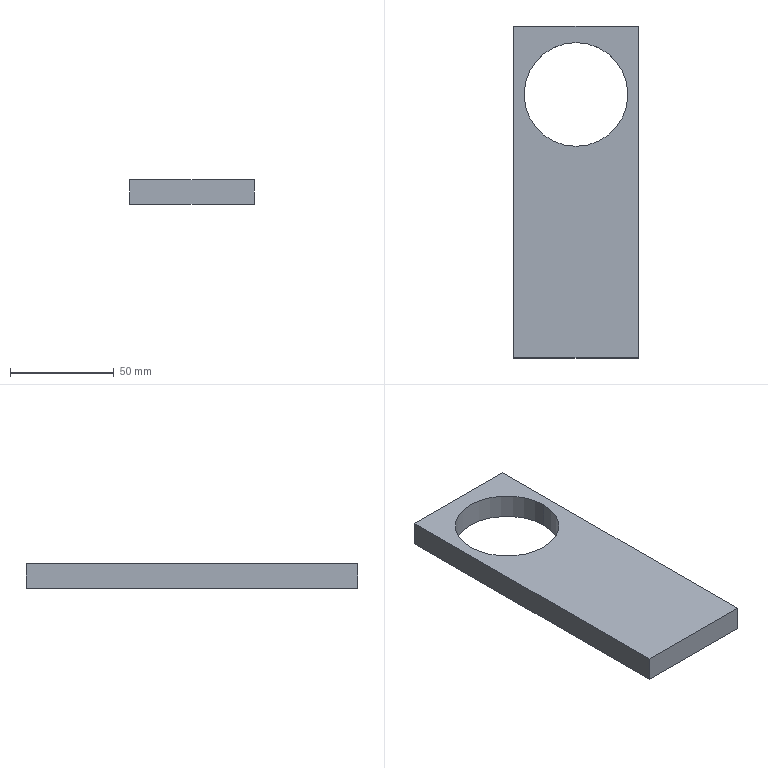Part | SolidWorks | features Extrusion 1, ICE 1 | 1 solid | 8 faces | box 60 x 160 x 12 mm | volume 91638 mm3 | plane 6 | cylinder 2 | commonest cylinder face diameters 50 x2
STEP:
#1=CARTESIAN_POINT('',(-25.,47.,0.));
#2=VERTEX_POINT('',#1);
#3=CARTESIAN_POINT('',(25.,47.,0.));
#4=VERTEX_POINT('',#3);
#5=CARTESIAN_POINT('',(0.,47.,0.));
#6=DIRECTION('',(0.,0.,1.));
#7=DIRECTION('',(1.,0.,0.));
#8=AXIS2_PLACEMENT_3D('',#5,#6,#7);
#9=CIRCLE('',#8,25.);
#10=EDGE_CURVE('',#2,#4,#9,.T.);
#11=ORIENTED_EDGE('',*,*,#10,.F.);
#12=CARTESIAN_POINT('',(-25.,47.,12.));
#13=VERTEX_POINT('',#12);
#14=CARTESIAN_POINT('',(-25.,47.,0.));
#15=DIRECTION('',(0.,0.,1.));
#16=VECTOR('',#15,1000.);
#17=LINE('',#14,#16);
#18=EDGE_CURVE('',#2,#13,#17,.T.);
#19=ORIENTED_EDGE('',*,*,#18,.T.);
#20=CARTESIAN_POINT('',(25.,47.,12.));
#21=VERTEX_POINT('',#20);
#22=CARTESIAN_POINT('',(0.,47.,12.));
#23=DIRECTION('',(0.,0.,1.));
#24=DIRECTION('',(1.,0.,0.));
#25=AXIS2_PLACEMENT_3D('',#22,#23,#24);
#26=CIRCLE('',#25,25.);
#27=EDGE_CURVE('',#13,#21,#26,.T.);
#28=ORIENTED_EDGE('',*,*,#27,.T.);
#29=CARTESIAN_POINT('',(25.,47.,0.));
#30=DIRECTION('',(0.,0.,1.));
#31=VECTOR('',#30,1000.);
#32=LINE('',#29,#31);
#33=EDGE_CURVE('',#4,#21,#32,.T.);
#34=ORIENTED_EDGE('',*,*,#33,.F.);
#35=EDGE_LOOP('',(#11,#19,#28,#34));
#36=FACE_OUTER_BOUND('',#35,.T.);
#37=CARTESIAN_POINT('',(0.,47.,0.));
#38=DIRECTION('',(0.,0.,1.));
#39=DIRECTION('',(1.,0.,0.));
#40=AXIS2_PLACEMENT_3D('',#37,#38,#39);
#41=CYLINDRICAL_SURFACE('',#40,25.);
#42=ADVANCED_FACE('',(#36),#41,.F.);
#43=CARTESIAN_POINT('',(30.,-80.,0.));
#44=VERTEX_POINT('',#43);
#45=CARTESIAN_POINT('',(30.,80.,0.));
#46=VERTEX_POINT('',#45);
#47=CARTESIAN_POINT('',(30.,-80.,0.));
#48=DIRECTION('',(0.,1.,0.));
#49=VECTOR('',#48,1000.);
#50=LINE('',#47,#49);
#51=EDGE_CURVE('',#44,#46,#50,.T.);
#52=ORIENTED_EDGE('',*,*,#51,.T.);
#53=CARTESIAN_POINT('',(30.,80.,12.));
#54=VERTEX_POINT('',#53);
#55=CARTESIAN_POINT('',(30.,80.,12.));
#56=DIRECTION('',(0.,0.,-1.));
#57=VECTOR('',#56,1000.);
#58=LINE('',#55,#57);
#59=EDGE_CURVE('',#54,#46,#58,.T.);
#60=ORIENTED_EDGE('',*,*,#59,.F.);
#61=CARTESIAN_POINT('',(30.,-80.,12.));
#62=VERTEX_POINT('',#61);
#63=CARTESIAN_POINT('',(30.,-80.,12.));
#64=DIRECTION('',(0.,1.,0.));
#65=VECTOR('',#64,1000.);
#66=LINE('',#63,#65);
#67=EDGE_CURVE('',#62,#54,#66,.T.);
#68=ORIENTED_EDGE('',*,*,#67,.F.);
#69=CARTESIAN_POINT('',(30.,-80.,12.));
#70=DIRECTION('',(0.,0.,-1.));
#71=VECTOR('',#70,1000.);
#72=LINE('',#69,#71);
#73=EDGE_CURVE('',#62,#44,#72,.T.);
#74=ORIENTED_EDGE('',*,*,#73,.T.);
#75=EDGE_LOOP('',(#52,#60,#68,#74));
#76=FACE_OUTER_BOUND('',#75,.T.);
#77=CARTESIAN_POINT('',(30.,-80.,12.));
#78=DIRECTION('',(-1.,0.,0.));
#79=DIRECTION('',(0.,0.,1.));
#80=AXIS2_PLACEMENT_3D('',#77,#78,#79);
#81=PLANE('',#80);
#82=ADVANCED_FACE('',(#76),#81,.F.);
#83=CARTESIAN_POINT('',(-30.,80.,0.));
#84=VERTEX_POINT('',#83);
#85=CARTESIAN_POINT('',(-30.,80.,0.));
#86=DIRECTION('',(-1.,0.,0.));
#87=VECTOR('',#86,1000.);
#88=LINE('',#85,#87);
#89=EDGE_CURVE('',#46,#84,#88,.T.);
#90=ORIENTED_EDGE('',*,*,#89,.T.);
#91=CARTESIAN_POINT('',(-30.,80.,12.));
#92=VERTEX_POINT('',#91);
#93=CARTESIAN_POINT('',(-30.,80.,12.));
#94=DIRECTION('',(0.,0.,-1.));
#95=VECTOR('',#94,1000.);
#96=LINE('',#93,#95);
#97=EDGE_CURVE('',#92,#84,#96,.T.);
#98=ORIENTED_EDGE('',*,*,#97,.F.);
#99=CARTESIAN_POINT('',(-30.,80.,12.));
#100=DIRECTION('',(-1.,0.,0.));
#101=VECTOR('',#100,1000.);
#102=LINE('',#99,#101);
#103=EDGE_CURVE('',#54,#92,#102,.T.);
#104=ORIENTED_EDGE('',*,*,#103,.F.);
#105=ORIENTED_EDGE('',*,*,#59,.T.);
#106=EDGE_LOOP('',(#90,#98,#104,#105));
#107=FACE_OUTER_BOUND('',#106,.T.);
#108=CARTESIAN_POINT('',(-30.,80.,12.));
#109=DIRECTION('',(0.,-1.,0.));
#110=DIRECTION('',(0.,0.,-1.));
#111=AXIS2_PLACEMENT_3D('',#108,#109,#110);
#112=PLANE('',#111);
#113=ADVANCED_FACE('',(#107),#112,.F.);
#114=CARTESIAN_POINT('',(-30.,-80.,0.));
#115=VERTEX_POINT('',#114);
#116=CARTESIAN_POINT('',(-30.,-80.,0.));
#117=DIRECTION('',(0.,-1.,0.));
#118=VECTOR('',#117,1000.);
#119=LINE('',#116,#118);
#120=EDGE_CURVE('',#84,#115,#119,.T.);
#121=ORIENTED_EDGE('',*,*,#120,.T.);
#122=CARTESIAN_POINT('',(-30.,-80.,12.));
#123=VERTEX_POINT('',#122);
#124=CARTESIAN_POINT('',(-30.,-80.,12.));
#125=DIRECTION('',(0.,0.,-1.));
#126=VECTOR('',#125,1000.);
#127=LINE('',#124,#126);
#128=EDGE_CURVE('',#123,#115,#127,.T.);
#129=ORIENTED_EDGE('',*,*,#128,.F.);
#130=CARTESIAN_POINT('',(-30.,-80.,12.));
#131=DIRECTION('',(0.,-1.,0.));
#132=VECTOR('',#131,1000.);
#133=LINE('',#130,#132);
#134=EDGE_CURVE('',#92,#123,#133,.T.);
#135=ORIENTED_EDGE('',*,*,#134,.F.);
#136=ORIENTED_EDGE('',*,*,#97,.T.);
#137=EDGE_LOOP('',(#121,#129,#135,#136));
#138=FACE_OUTER_BOUND('',#137,.T.);
#139=CARTESIAN_POINT('',(-30.,-80.,12.));
#140=DIRECTION('',(1.,0.,0.));
#141=DIRECTION('',(0.,0.,-1.));
#142=AXIS2_PLACEMENT_3D('',#139,#140,#141);
#143=PLANE('',#142);
#144=ADVANCED_FACE('',(#138),#143,.F.);
#145=CARTESIAN_POINT('',(-30.,-80.,0.));
#146=DIRECTION('',(1.,0.,0.));
#147=VECTOR('',#146,1000.);
#148=LINE('',#145,#147);
#149=EDGE_CURVE('',#115,#44,#148,.T.);
#150=ORIENTED_EDGE('',*,*,#149,.T.);
#151=ORIENTED_EDGE('',*,*,#73,.F.);
#152=CARTESIAN_POINT('',(-30.,-80.,12.));
#153=DIRECTION('',(1.,0.,0.));
#154=VECTOR('',#153,1000.);
#155=LINE('',#152,#154);
#156=EDGE_CURVE('',#123,#62,#155,.T.);
#157=ORIENTED_EDGE('',*,*,#156,.F.);
#158=ORIENTED_EDGE('',*,*,#128,.T.);
#159=EDGE_LOOP('',(#150,#151,#157,#158));
#160=FACE_OUTER_BOUND('',#159,.T.);
#161=CARTESIAN_POINT('',(-30.,-80.,12.));
#162=DIRECTION('',(0.,1.,0.));
#163=DIRECTION('',(0.,0.,1.));
#164=AXIS2_PLACEMENT_3D('',#161,#162,#163);
#165=PLANE('',#164);
#166=ADVANCED_FACE('',(#160),#165,.F.);
#167=CARTESIAN_POINT('',(0.,47.,12.));
#168=DIRECTION('',(0.,0.,1.));
#169=DIRECTION('',(1.,0.,0.));
#170=AXIS2_PLACEMENT_3D('',#167,#168,#169);
#171=CIRCLE('',#170,25.);
#172=EDGE_CURVE('',#21,#13,#171,.T.);
#173=ORIENTED_EDGE('',*,*,#172,.F.);
#174=ORIENTED_EDGE('',*,*,#27,.F.);
#175=EDGE_LOOP('',(#173,#174));
#176=FACE_BOUND('',#175,.T.);
#177=ORIENTED_EDGE('',*,*,#67,.T.);
#178=ORIENTED_EDGE('',*,*,#103,.T.);
#179=ORIENTED_EDGE('',*,*,#134,.T.);
#180=ORIENTED_EDGE('',*,*,#156,.T.);
#181=EDGE_LOOP('',(#177,#178,#179,#180));
#182=FACE_OUTER_BOUND('',#181,.T.);
#183=CARTESIAN_POINT('',(0.,0.,12.));
#184=DIRECTION('',(0.,0.,-1.));
#185=DIRECTION('',(-1.,0.,0.));
#186=AXIS2_PLACEMENT_3D('',#183,#184,#185);
#187=PLANE('',#186);
#188=ADVANCED_FACE('',(#176,#182),#187,.F.);
#189=CARTESIAN_POINT('',(0.,47.,0.));
#190=DIRECTION('',(0.,0.,1.));
#191=DIRECTION('',(1.,0.,0.));
#192=AXIS2_PLACEMENT_3D('',#189,#190,#191);
#193=CIRCLE('',#192,25.);
#194=EDGE_CURVE('',#4,#2,#193,.T.);
#195=ORIENTED_EDGE('',*,*,#194,.T.);
#196=ORIENTED_EDGE('',*,*,#10,.T.);
#197=EDGE_LOOP('',(#195,#196));
#198=FACE_BOUND('',#197,.T.);
#199=ORIENTED_EDGE('',*,*,#51,.F.);
#200=ORIENTED_EDGE('',*,*,#149,.F.);
#201=ORIENTED_EDGE('',*,*,#120,.F.);
#202=ORIENTED_EDGE('',*,*,#89,.F.);
#203=EDGE_LOOP('',(#199,#200,#201,#202));
#204=FACE_OUTER_BOUND('',#203,.T.);
#205=CARTESIAN_POINT('',(0.,0.,0.));
#206=DIRECTION('',(0.,0.,-1.));
#207=DIRECTION('',(-1.,0.,0.));
#208=AXIS2_PLACEMENT_3D('',#205,#206,#207);
#209=PLANE('',#208);
#210=ADVANCED_FACE('',(#198,#204),#209,.T.);
#211=ORIENTED_EDGE('',*,*,#18,.F.);
#212=ORIENTED_EDGE('',*,*,#194,.F.);
#213=ORIENTED_EDGE('',*,*,#33,.T.);
#214=ORIENTED_EDGE('',*,*,#172,.T.);
#215=EDGE_LOOP('',(#211,#212,#213,#214));
#216=FACE_OUTER_BOUND('',#215,.T.);
#217=CARTESIAN_POINT('',(0.,47.,0.));
#218=DIRECTION('',(0.,0.,1.));
#219=DIRECTION('',(1.,0.,0.));
#220=AXIS2_PLACEMENT_3D('',#217,#218,#219);
#221=CYLINDRICAL_SURFACE('',#220,25.);
#222=ADVANCED_FACE('',(#216),#221,.F.);
#223=CLOSED_SHELL('',(#42,#82,#113,#144,#166,#188,#210,#222));
#224=MANIFOLD_SOLID_BREP('',#223);
#225=CARTESIAN_POINT('',(0.,0.,0.));
#226=DIRECTION('',(0.,0.,1.));
#227=DIRECTION('',(1.,0.,0.));
#228=AXIS2_PLACEMENT_3D('',#225,#226,#227);
#229=(LENGTH_UNIT()NAMED_UNIT(*)SI_UNIT(.MILLI.,.METRE.));
#230=UNCERTAINTY_MEASURE_WITH_UNIT(LENGTH_MEASURE(0.00001),#229,'','');
#231=(NAMED_UNIT(*)PLANE_ANGLE_UNIT()SI_UNIT($,.RADIAN.));
#232=(NAMED_UNIT(*)SI_UNIT($,.STERADIAN.)SOLID_ANGLE_UNIT());
#233=(GEOMETRIC_REPRESENTATION_CONTEXT(3)GLOBAL_UNCERTAINTY_ASSIGNED_CONTEXT((#230))GLOBAL_UNIT_ASSIGNED_CONTEXT((#229,#231,#232))REPRESENTATION_CONTEXT('',''));
#234=ADVANCED_BREP_SHAPE_REPRESENTATION('',(#224,#228),#233);